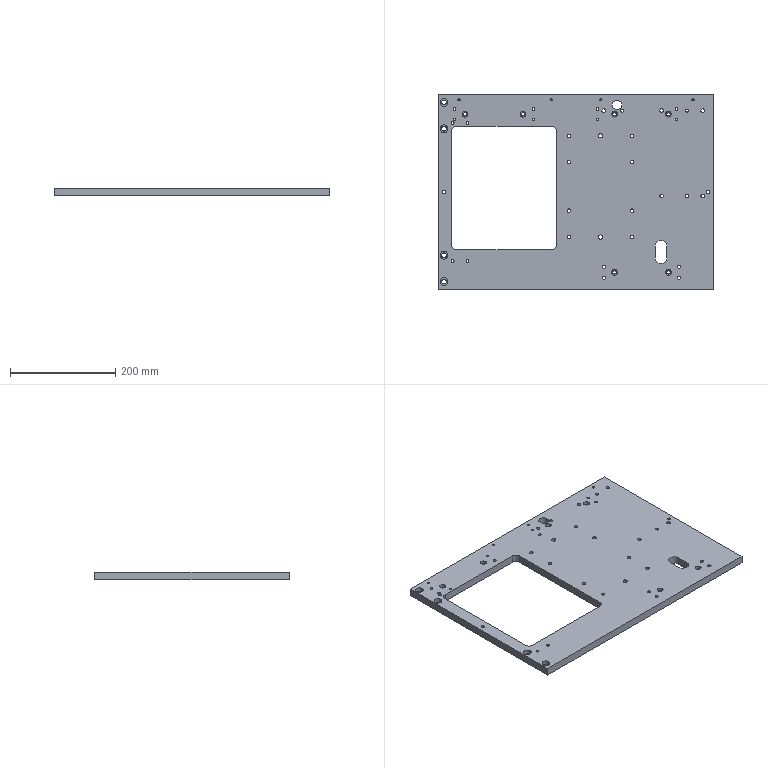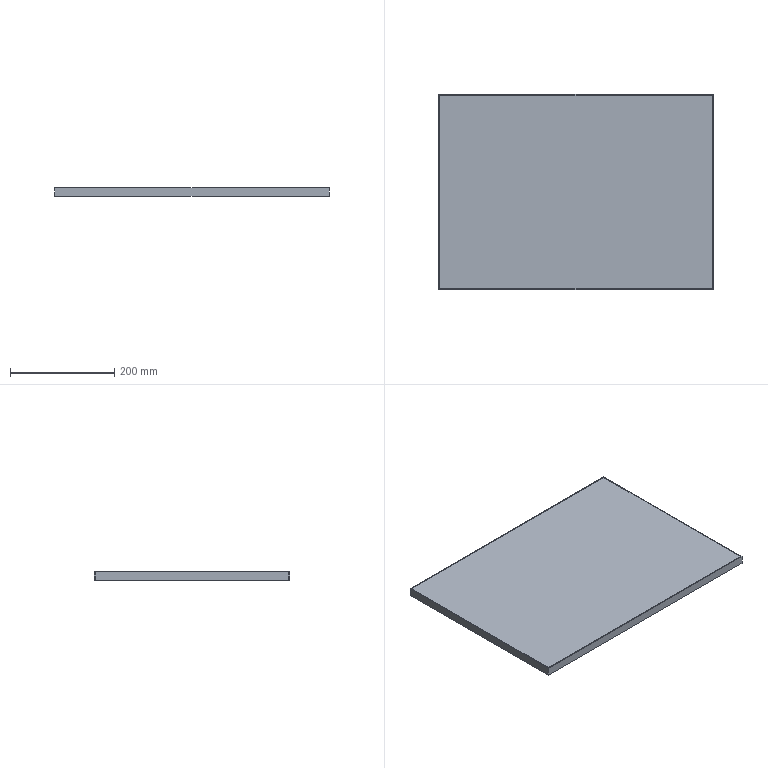CAM job | NX | 3-axis milling, drilling | part box 521 x 370 x 15 mm | stock box 525 x 374 x 16 mm
Tools:
number,name,description,diameter,corner_radius,flute_length,length,flutes
1,D50,Milling Tool-5 Parameters,50.0,0.0,50.0,75.0,2
3,D10,Milling Tool-5 Parameters,10.0,0.0,50.0,75.0,2
2,D6A45,Milling Tool-5 Parameters,6.0,0.0,3.0,3.0,2
15,5.0ZT,Drilling Tool,5.0,0.0,35.0,50.0,2
17,5.8ZT,Drilling Tool,5.8,0.0,35.0,50.0,2
16,6.0JD,Milling Tool-5 Parameters,6.0,0.0,30.0,30.0,4
19,9.0ZT,Drilling Tool,9.0,0.0,35.0,50.0,2
11,6.6ZT,Drilling Tool,6.6,0.0,35.0,50.0,2
12,6.8ZT,Drilling Tool,6.8,0.0,35.0,50.0,2
13,M8,Milling Tool-5 Parameters,6.8,0.0,30.0,30.0,4
14,7.8ZT,Drilling Tool,7.8,0.0,35.0,50.0,2
24,8.0JD,Milling Tool-5 Parameters,8.0,0.0,30.0,30.0,4
22,3.3ZT,Drilling Tool,3.3,0.0,35.0,50.0,2
23,M4,Milling Tool-5 Parameters,3.3,0.0,30.0,30.0,4
4,D10JING,Milling Tool-5 Parameters,10.0,0.0,50.0,75.0,2
8,D6,Milling Tool-5 Parameters,6.0,0.0,50.0,75.0,2
Operations:
program,operation,operation_type,tool,method,geometry_group,spindle_rpm,surface_speed,feed_per_tooth,feed_cut,feed_plunge,cut_length_mm,path_length_mm,cut_time_min,machine_time_min
1-524-373-15毛胚-AB胶,FLOOR_WALL,VolumeBased25DMillingOperation,D50,METHOD,A,6500.0,1286.0,0.0962,1250.0,100.0,9565.996,9619.996,7.653,7.658
1-524-373-15毛胚-AB胶,DRILLING_COPY_1,Operation,D6A45,METHOD,A,3000.0,56.0,0.0333,200.0,0.0,234.6,2860.423,1.173,1.436
1-524-373-15毛胚-AB胶,DRILLING_COPY_1_COPY,Operation,5.0ZT,METHOD,A,2000.0,15.0,0.0375,150.0,0.0,252.026,1409.079,1.68,1.796
1-524-373-15毛胚-AB胶,DRILLING_COPY_1_COPY_COPY,Operation,5.8ZT,METHOD,A,2000.0,15.0,0.0375,150.0,0.0,191.183,1444.951,1.274,1.4
1-524-373-15毛胚-AB胶,DRILLING_COPY_1_COPY_COPY_COPY,Operation,6.0JD,METHOD,A,1000.0,18.0,0.0125,50.0,0.0,166.5,1395.587,3.33,3.453
1-524-373-15毛胚-AB胶,DRILLING_COPY_1_COPY_COPY_COPY_1,Operation,9.0ZT,METHOD,A,2000.0,15.0,0.0375,150.0,0.0,88.816,586.83,0.5921,0.6419
1-524-373-15毛胚-AB胶,DRILLING_COPY_1_COPY_COPY_1_COPY_1,Operation,6.6ZT,METHOD,A,2000.0,18.0,0.03,120.0,0.0,128.897,1120.764,1.074,1.173
1-524-373-15毛胚-AB胶,DRILLING_COPY_1_COPY_COPY_1_COPY_1_COPY,Operation,6.8ZT,METHOD,A,2000.0,18.0,0.03,120.0,0.0,280.058,1554.118,2.334,2.461
1-524-373-15毛胚-AB胶,DRILLING_COPY_1_COPY_COPY_1_COPY_1_COPY_COPY,Operation,M8,METHOD,A,200.0,4.0,0.3125,250.0,0.0,240.5,1475.002,0.962,1.085
1-524-373-15毛胚-AB胶,DRILLING_COPY_1_COPY_COPY_1_COPY_1_COPY_COPY_1,Operation,7.8ZT,METHOD,A,2000.0,18.0,0.03,120.0,0.0,43.687,342.397,0.3641,0.3939
1-524-373-15毛胚-AB胶,DRILLING_COPY_1_COPY_COPY_1_COPY_1_COPY_COPY_1_COPY,Operation,8.0JD,METHOD,A,1000.0,25.0,0.0125,50.0,0.0,37.0,329.023,0.74,0.7692
1-524-373-15毛胚-AB胶,DRILLING_COPY_1_COPY_COPY_COPY_COPY_COPY_COPY_1,Operation,3.3ZT,METHOD,A,2000.0,20.0,0.0375,150.0,0.0,81.966,677.031,0.5464,0.6059
1-524-373-15毛胚-AB胶,DRILLING_COPY_1_COPY_COPY_COPY_COPY_COPY_COPY,Operation,M4,METHOD,A,200.0,2.0,0.175,140.0,0.0,74.0,661.099,0.5286,0.5873
1-524-373-15毛胚-AB胶,ZLEVEL_PROFILE,ZLevelMilling,D10,METHOD,A,7000.0,219.0,0.2143,3000.0,1000.0,27314.283,27385.683,9.136,9.143
1-524-373-15毛胚-AB胶,ZLEVEL_PROFILE_COPY,ZLevelMilling,D10,METHOD,A,7000.0,219.0,0.2143,3000.0,1000.0,14170.772,15060.522,4.818,4.907
1-524-373-15毛胚-AB胶,HOLE_MILLING,CylinderMilling,D10JING,METHOD,A,7000.0,131.0,0.1071,1500.0,100.0,809.886,1422.286,0.5399,0.6012
1-524-373-15毛胚-AB胶,HOLE_MILLING_1,CylinderMilling,D6,METHOD,A,7000.0,131.0,0.1071,1500.0,100.0,1442.65,2625.85,0.9618,1.08
1-524-373-15毛胚-AB胶,ZLEVEL_PROFILE_COPY_COPY_1_COPY_COPY_COPY_1,ZLevelMilling,D6,METHOD,A,7000.0,219.0,0.0714,1000.0,100.0,972.052,1870.704,0.9721,1.062
1-524-373-15毛胚-AB胶,ZLEVEL_PROFILE_COPY_1_COPY_COPY_COPY_COPY_2_COPY,ZLevelMilling,D6A45,METHOD,A,7000.0,131.0,0.0714,1000.0,1000.0,3801.328,19759.088,3.801,5.397
1-524-373-15毛胚-AB胶,ZLEVEL_PROFILE_COPY_1_1,ZLevelMilling,D10JING,METHOD,A,7000.0,219.0,0.0714,1000.0,1000.0,5673.491,5750.241,5.673,5.681
2-524-373-15毛胚-AB胶,FLOOR_WALL_COPY,VolumeBased25DMillingOperation,D50,METHOD,B,6500.0,1286.0,0.0962,1250.0,100.0,8926.997,8980.997,7.142,7.147
2-524-373-15毛胚-AB胶,ZLEVEL_PROFILE_COPY_1_COPY_COPY_COPY_COPY_2_COPY_COPY,ZLevelMilling,D6A45,METHOD,B,7000.0,131.0,0.0714,1000.0,1000.0,3631.446,19333.132,3.631,5.202